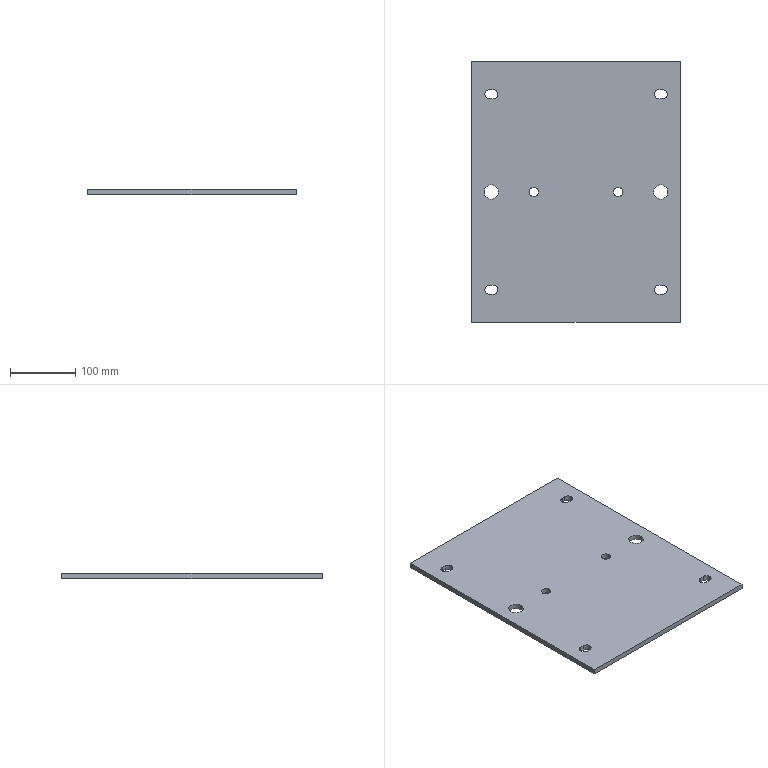Part | 1 solid | 34 faces | box 320 x 400 x 8 mm | volume 1007841 mm3 | cylinder 20 | plane 14 | commonest cylinder face diameters 14 x16 22 x4
STEP:
#1=CARTESIAN_POINT('',(140.,150.,-8.));
#2=VERTEX_POINT('',#1);
#3=CARTESIAN_POINT('',(133.,157.,-8.));
#4=VERTEX_POINT('',#3);
#5=CARTESIAN_POINT('',(133.,150.,-8.));
#6=DIRECTION('',(0.,0.,1.));
#7=DIRECTION('',(1.,0.,0.));
#8=AXIS2_PLACEMENT_3D('',#5,#6,#7);
#9=CIRCLE('',#8,7.);
#10=EDGE_CURVE('',#2,#4,#9,.T.);
#11=ORIENTED_EDGE('',*,*,#10,.F.);
#12=CARTESIAN_POINT('',(140.,150.,0.));
#13=VERTEX_POINT('',#12);
#14=CARTESIAN_POINT('',(140.,150.,-10.));
#15=DIRECTION('',(0.,0.,1.));
#16=VECTOR('',#15,1000.);
#17=LINE('',#14,#16);
#18=EDGE_CURVE('',#2,#13,#17,.T.);
#19=ORIENTED_EDGE('',*,*,#18,.T.);
#20=CARTESIAN_POINT('',(133.,157.,0.));
#21=VERTEX_POINT('',#20);
#22=CARTESIAN_POINT('',(133.,150.,0.));
#23=DIRECTION('',(0.,0.,1.));
#24=DIRECTION('',(-1.,0.,0.));
#25=AXIS2_PLACEMENT_3D('',#22,#23,#24);
#26=CIRCLE('',#25,7.);
#27=EDGE_CURVE('',#13,#21,#26,.T.);
#28=ORIENTED_EDGE('',*,*,#27,.T.);
#29=CARTESIAN_POINT('',(133.,157.,-10.));
#30=DIRECTION('',(0.,0.,1.));
#31=VECTOR('',#30,1000.);
#32=LINE('',#29,#31);
#33=EDGE_CURVE('',#4,#21,#32,.T.);
#34=ORIENTED_EDGE('',*,*,#33,.F.);
#35=EDGE_LOOP('',(#11,#19,#28,#34));
#36=FACE_OUTER_BOUND('',#35,.T.);
#37=CARTESIAN_POINT('',(133.,150.,-10.));
#38=DIRECTION('',(0.,0.,1.));
#39=DIRECTION('',(1.,0.,0.));
#40=AXIS2_PLACEMENT_3D('',#37,#38,#39);
#41=CYLINDRICAL_SURFACE('',#40,7.);
#42=ADVANCED_FACE('',(#36),#41,.F.);
#43=CARTESIAN_POINT('',(119.,0.,-8.));
#44=VERTEX_POINT('',#43);
#45=CARTESIAN_POINT('',(141.,0.,-8.));
#46=VERTEX_POINT('',#45);
#47=CARTESIAN_POINT('',(130.,0.,-8.));
#48=DIRECTION('',(0.,0.,1.));
#49=DIRECTION('',(1.,0.,0.));
#50=AXIS2_PLACEMENT_3D('',#47,#48,#49);
#51=CIRCLE('',#50,11.);
#52=EDGE_CURVE('',#44,#46,#51,.T.);
#53=ORIENTED_EDGE('',*,*,#52,.F.);
#54=CARTESIAN_POINT('',(119.,0.,0.));
#55=VERTEX_POINT('',#54);
#56=CARTESIAN_POINT('',(119.,0.,-10.));
#57=DIRECTION('',(0.,0.,1.));
#58=VECTOR('',#57,1000.);
#59=LINE('',#56,#58);
#60=EDGE_CURVE('',#44,#55,#59,.T.);
#61=ORIENTED_EDGE('',*,*,#60,.T.);
#62=CARTESIAN_POINT('',(141.,0.,0.));
#63=VERTEX_POINT('',#62);
#64=CARTESIAN_POINT('',(130.,0.,0.));
#65=DIRECTION('',(0.,0.,1.));
#66=DIRECTION('',(-1.,0.,0.));
#67=AXIS2_PLACEMENT_3D('',#64,#65,#66);
#68=CIRCLE('',#67,11.);
#69=EDGE_CURVE('',#55,#63,#68,.T.);
#70=ORIENTED_EDGE('',*,*,#69,.T.);
#71=CARTESIAN_POINT('',(141.,0.,-10.));
#72=DIRECTION('',(0.,0.,1.));
#73=VECTOR('',#72,1000.);
#74=LINE('',#71,#73);
#75=EDGE_CURVE('',#46,#63,#74,.T.);
#76=ORIENTED_EDGE('',*,*,#75,.F.);
#77=EDGE_LOOP('',(#53,#61,#70,#76));
#78=FACE_OUTER_BOUND('',#77,.T.);
#79=CARTESIAN_POINT('',(130.,0.,-10.));
#80=DIRECTION('',(0.,0.,1.));
#81=DIRECTION('',(1.,0.,0.));
#82=AXIS2_PLACEMENT_3D('',#79,#80,#81);
#83=CYLINDRICAL_SURFACE('',#82,11.);
#84=ADVANCED_FACE('',(#78),#83,.F.);
#85=CARTESIAN_POINT('',(140.,-150.,-8.));
#86=VERTEX_POINT('',#85);
#87=CARTESIAN_POINT('',(133.,-143.,-8.));
#88=VERTEX_POINT('',#87);
#89=CARTESIAN_POINT('',(133.,-150.,-8.));
#90=DIRECTION('',(0.,0.,1.));
#91=DIRECTION('',(1.,0.,0.));
#92=AXIS2_PLACEMENT_3D('',#89,#90,#91);
#93=CIRCLE('',#92,7.);
#94=EDGE_CURVE('',#86,#88,#93,.T.);
#95=ORIENTED_EDGE('',*,*,#94,.F.);
#96=CARTESIAN_POINT('',(140.,-150.,0.));
#97=VERTEX_POINT('',#96);
#98=CARTESIAN_POINT('',(140.,-150.,-10.));
#99=DIRECTION('',(0.,0.,1.));
#100=VECTOR('',#99,1000.);
#101=LINE('',#98,#100);
#102=EDGE_CURVE('',#86,#97,#101,.T.);
#103=ORIENTED_EDGE('',*,*,#102,.T.);
#104=CARTESIAN_POINT('',(133.,-143.,0.));
#105=VERTEX_POINT('',#104);
#106=CARTESIAN_POINT('',(133.,-150.,0.));
#107=DIRECTION('',(0.,0.,1.));
#108=DIRECTION('',(1.,0.,0.));
#109=AXIS2_PLACEMENT_3D('',#106,#107,#108);
#110=CIRCLE('',#109,7.);
#111=EDGE_CURVE('',#97,#105,#110,.T.);
#112=ORIENTED_EDGE('',*,*,#111,.T.);
#113=CARTESIAN_POINT('',(133.,-143.,-10.));
#114=DIRECTION('',(0.,0.,1.));
#115=VECTOR('',#114,1000.);
#116=LINE('',#113,#115);
#117=EDGE_CURVE('',#88,#105,#116,.T.);
#118=ORIENTED_EDGE('',*,*,#117,.F.);
#119=EDGE_LOOP('',(#95,#103,#112,#118));
#120=FACE_OUTER_BOUND('',#119,.T.);
#121=CARTESIAN_POINT('',(133.,-150.,-10.));
#122=DIRECTION('',(0.,0.,1.));
#123=DIRECTION('',(1.,0.,0.));
#124=AXIS2_PLACEMENT_3D('',#121,#122,#123);
#125=CYLINDRICAL_SURFACE('',#124,7.);
#126=ADVANCED_FACE('',(#120),#125,.F.);
#127=CARTESIAN_POINT('',(-141.,0.,-8.));
#128=VERTEX_POINT('',#127);
#129=CARTESIAN_POINT('',(-119.,0.,-8.));
#130=VERTEX_POINT('',#129);
#131=CARTESIAN_POINT('',(-130.,0.,-8.));
#132=DIRECTION('',(0.,0.,1.));
#133=DIRECTION('',(1.,0.,0.));
#134=AXIS2_PLACEMENT_3D('',#131,#132,#133);
#135=CIRCLE('',#134,11.);
#136=EDGE_CURVE('',#128,#130,#135,.T.);
#137=ORIENTED_EDGE('',*,*,#136,.F.);
#138=CARTESIAN_POINT('',(-141.,0.,0.));
#139=VERTEX_POINT('',#138);
#140=CARTESIAN_POINT('',(-141.,0.,-10.));
#141=DIRECTION('',(0.,0.,1.));
#142=VECTOR('',#141,1000.);
#143=LINE('',#140,#142);
#144=EDGE_CURVE('',#128,#139,#143,.T.);
#145=ORIENTED_EDGE('',*,*,#144,.T.);
#146=CARTESIAN_POINT('',(-119.,0.,0.));
#147=VERTEX_POINT('',#146);
#148=CARTESIAN_POINT('',(-130.,0.,0.));
#149=DIRECTION('',(0.,0.,1.));
#150=DIRECTION('',(1.,0.,0.));
#151=AXIS2_PLACEMENT_3D('',#148,#149,#150);
#152=CIRCLE('',#151,11.);
#153=EDGE_CURVE('',#139,#147,#152,.T.);
#154=ORIENTED_EDGE('',*,*,#153,.T.);
#155=CARTESIAN_POINT('',(-119.,0.,-10.));
#156=DIRECTION('',(0.,0.,1.));
#157=VECTOR('',#156,1000.);
#158=LINE('',#155,#157);
#159=EDGE_CURVE('',#130,#147,#158,.T.);
#160=ORIENTED_EDGE('',*,*,#159,.F.);
#161=EDGE_LOOP('',(#137,#145,#154,#160));
#162=FACE_OUTER_BOUND('',#161,.T.);
#163=CARTESIAN_POINT('',(-130.,0.,-10.));
#164=DIRECTION('',(0.,0.,1.));
#165=DIRECTION('',(1.,0.,0.));
#166=AXIS2_PLACEMENT_3D('',#163,#164,#165);
#167=CYLINDRICAL_SURFACE('',#166,11.);
#168=ADVANCED_FACE('',(#162),#167,.F.);
#169=CARTESIAN_POINT('',(-120.,150.,-8.));
#170=VERTEX_POINT('',#169);
#171=CARTESIAN_POINT('',(-127.,157.,-8.));
#172=VERTEX_POINT('',#171);
#173=CARTESIAN_POINT('',(-127.,150.,-8.));
#174=DIRECTION('',(0.,0.,1.));
#175=DIRECTION('',(1.,0.,0.));
#176=AXIS2_PLACEMENT_3D('',#173,#174,#175);
#177=CIRCLE('',#176,7.);
#178=EDGE_CURVE('',#170,#172,#177,.T.);
#179=ORIENTED_EDGE('',*,*,#178,.F.);
#180=CARTESIAN_POINT('',(-120.,150.,0.));
#181=VERTEX_POINT('',#180);
#182=CARTESIAN_POINT('',(-120.,150.,-10.));
#183=DIRECTION('',(0.,0.,1.));
#184=VECTOR('',#183,1000.);
#185=LINE('',#182,#184);
#186=EDGE_CURVE('',#170,#181,#185,.T.);
#187=ORIENTED_EDGE('',*,*,#186,.T.);
#188=CARTESIAN_POINT('',(-127.,157.,0.));
#189=VERTEX_POINT('',#188);
#190=CARTESIAN_POINT('',(-127.,150.,0.));
#191=DIRECTION('',(0.,0.,1.));
#192=DIRECTION('',(1.,0.,0.));
#193=AXIS2_PLACEMENT_3D('',#190,#191,#192);
#194=CIRCLE('',#193,7.);
#195=EDGE_CURVE('',#181,#189,#194,.T.);
#196=ORIENTED_EDGE('',*,*,#195,.T.);
#197=CARTESIAN_POINT('',(-127.,157.,-10.));
#198=DIRECTION('',(0.,0.,1.));
#199=VECTOR('',#198,1000.);
#200=LINE('',#197,#199);
#201=EDGE_CURVE('',#172,#189,#200,.T.);
#202=ORIENTED_EDGE('',*,*,#201,.F.);
#203=EDGE_LOOP('',(#179,#187,#196,#202));
#204=FACE_OUTER_BOUND('',#203,.T.);
#205=CARTESIAN_POINT('',(-127.,150.,-10.));
#206=DIRECTION('',(0.,0.,1.));
#207=DIRECTION('',(1.,0.,0.));
#208=AXIS2_PLACEMENT_3D('',#205,#206,#207);
#209=CYLINDRICAL_SURFACE('',#208,7.);
#210=ADVANCED_FACE('',(#204),#209,.F.);
#211=CARTESIAN_POINT('',(-120.,-150.,-8.));
#212=VERTEX_POINT('',#211);
#213=CARTESIAN_POINT('',(-127.,-143.,-8.));
#214=VERTEX_POINT('',#213);
#215=CARTESIAN_POINT('',(-127.,-150.,-8.));
#216=DIRECTION('',(0.,0.,1.));
#217=DIRECTION('',(1.,0.,0.));
#218=AXIS2_PLACEMENT_3D('',#215,#216,#217);
#219=CIRCLE('',#218,7.);
#220=EDGE_CURVE('',#212,#214,#219,.T.);
#221=ORIENTED_EDGE('',*,*,#220,.F.);
#222=CARTESIAN_POINT('',(-120.,-150.,0.));
#223=VERTEX_POINT('',#222);
#224=CARTESIAN_POINT('',(-120.,-150.,-10.));
#225=DIRECTION('',(0.,0.,1.));
#226=VECTOR('',#225,1000.);
#227=LINE('',#224,#226);
#228=EDGE_CURVE('',#212,#223,#227,.T.);
#229=ORIENTED_EDGE('',*,*,#228,.T.);
#230=CARTESIAN_POINT('',(-127.,-143.,0.));
#231=VERTEX_POINT('',#230);
#232=CARTESIAN_POINT('',(-127.,-150.,0.));
#233=DIRECTION('',(0.,0.,1.));
#234=DIRECTION('',(-1.,0.,0.));
#235=AXIS2_PLACEMENT_3D('',#232,#233,#234);
#236=CIRCLE('',#235,7.);
#237=EDGE_CURVE('',#223,#231,#236,.T.);
#238=ORIENTED_EDGE('',*,*,#237,.T.);
#239=CARTESIAN_POINT('',(-127.,-143.,-10.));
#240=DIRECTION('',(0.,0.,1.));
#241=VECTOR('',#240,1000.);
#242=LINE('',#239,#241);
#243=EDGE_CURVE('',#214,#231,#242,.T.);
#244=ORIENTED_EDGE('',*,*,#243,.F.);
#245=EDGE_LOOP('',(#221,#229,#238,#244));
#246=FACE_OUTER_BOUND('',#245,.T.);
#247=CARTESIAN_POINT('',(-127.,-150.,-10.));
#248=DIRECTION('',(0.,0.,1.));
#249=DIRECTION('',(1.,0.,0.));
#250=AXIS2_PLACEMENT_3D('',#247,#248,#249);
#251=CYLINDRICAL_SURFACE('',#250,7.);
#252=ADVANCED_FACE('',(#246),#251,.F.);
#253=CARTESIAN_POINT('',(58.,0.,-8.));
#254=VERTEX_POINT('',#253);
#255=CARTESIAN_POINT('',(72.,0.,-8.));
#256=VERTEX_POINT('',#255);
#257=CARTESIAN_POINT('',(65.,0.,-8.));
#258=DIRECTION('',(0.,0.,1.));
#259=DIRECTION('',(1.,0.,0.));
#260=AXIS2_PLACEMENT_3D('',#257,#258,#259);
#261=CIRCLE('',#260,7.);
#262=EDGE_CURVE('',#254,#256,#261,.T.);
#263=ORIENTED_EDGE('',*,*,#262,.F.);
#264=CARTESIAN_POINT('',(58.,0.,0.));
#265=VERTEX_POINT('',#264);
#266=CARTESIAN_POINT('',(58.,0.,-10.));
#267=DIRECTION('',(0.,0.,1.));
#268=VECTOR('',#267,1000.);
#269=LINE('',#266,#268);
#270=EDGE_CURVE('',#254,#265,#269,.T.);
#271=ORIENTED_EDGE('',*,*,#270,.T.);
#272=CARTESIAN_POINT('',(72.,0.,0.));
#273=VERTEX_POINT('',#272);
#274=CARTESIAN_POINT('',(65.,0.,0.));
#275=DIRECTION('',(0.,0.,1.));
#276=DIRECTION('',(-1.,0.,0.));
#277=AXIS2_PLACEMENT_3D('',#274,#275,#276);
#278=CIRCLE('',#277,7.);
#279=EDGE_CURVE('',#265,#273,#278,.T.);
#280=ORIENTED_EDGE('',*,*,#279,.T.);
#281=CARTESIAN_POINT('',(72.,0.,-10.));
#282=DIRECTION('',(0.,0.,1.));
#283=VECTOR('',#282,1000.);
#284=LINE('',#281,#283);
#285=EDGE_CURVE('',#256,#273,#284,.T.);
#286=ORIENTED_EDGE('',*,*,#285,.F.);
#287=EDGE_LOOP('',(#263,#271,#280,#286));
#288=FACE_OUTER_BOUND('',#287,.T.);
#289=CARTESIAN_POINT('',(65.,0.,-10.));
#290=DIRECTION('',(0.,0.,1.));
#291=DIRECTION('',(1.,0.,0.));
#292=AXIS2_PLACEMENT_3D('',#289,#290,#291);
#293=CYLINDRICAL_SURFACE('',#292,7.);
#294=ADVANCED_FACE('',(#288),#293,.F.);
#295=CARTESIAN_POINT('',(-72.,0.,-8.));
#296=VERTEX_POINT('',#295);
#297=CARTESIAN_POINT('',(-58.,0.,-8.));
#298=VERTEX_POINT('',#297);
#299=CARTESIAN_POINT('',(-65.,0.,-8.));
#300=DIRECTION('',(0.,0.,1.));
#301=DIRECTION('',(1.,0.,0.));
#302=AXIS2_PLACEMENT_3D('',#299,#300,#301);
#303=CIRCLE('',#302,7.);
#304=EDGE_CURVE('',#296,#298,#303,.T.);
#305=ORIENTED_EDGE('',*,*,#304,.F.);
#306=CARTESIAN_POINT('',(-72.,0.,0.));
#307=VERTEX_POINT('',#306);
#308=CARTESIAN_POINT('',(-72.,0.,-10.));
#309=DIRECTION('',(0.,0.,1.));
#310=VECTOR('',#309,1000.);
#311=LINE('',#308,#310);
#312=EDGE_CURVE('',#296,#307,#311,.T.);
#313=ORIENTED_EDGE('',*,*,#312,.T.);
#314=CARTESIAN_POINT('',(-58.,0.,0.));
#315=VERTEX_POINT('',#314);
#316=CARTESIAN_POINT('',(-65.,0.,0.));
#317=DIRECTION('',(0.,0.,1.));
#318=DIRECTION('',(1.,0.,0.));
#319=AXIS2_PLACEMENT_3D('',#316,#317,#318);
#320=CIRCLE('',#319,7.);
#321=EDGE_CURVE('',#307,#315,#320,.T.);
#322=ORIENTED_EDGE('',*,*,#321,.T.);
#323=CARTESIAN_POINT('',(-58.,0.,-10.));
#324=DIRECTION('',(0.,0.,1.));
#325=VECTOR('',#324,1000.);
#326=LINE('',#323,#325);
#327=EDGE_CURVE('',#298,#315,#326,.T.);
#328=ORIENTED_EDGE('',*,*,#327,.F.);
#329=EDGE_LOOP('',(#305,#313,#322,#328));
#330=FACE_OUTER_BOUND('',#329,.T.);
#331=CARTESIAN_POINT('',(-65.,0.,-10.));
#332=DIRECTION('',(0.,0.,1.));
#333=DIRECTION('',(1.,0.,0.));
#334=AXIS2_PLACEMENT_3D('',#331,#332,#333);
#335=CYLINDRICAL_SURFACE('',#334,7.);
#336=ADVANCED_FACE('',(#330),#335,.F.);
#337=CARTESIAN_POINT('',(160.,-200.,0.));
#338=VERTEX_POINT('',#337);
#339=CARTESIAN_POINT('',(160.,200.,0.));
#340=VERTEX_POINT('',#339);
#341=CARTESIAN_POINT('',(160.,200.,0.));
#342=DIRECTION('',(0.,1.,0.));
#343=VECTOR('',#342,1000.);
#344=LINE('',#341,#343);
#345=EDGE_CURVE('',#338,#340,#344,.T.);
#346=ORIENTED_EDGE('',*,*,#345,.F.);
#347=CARTESIAN_POINT('',(160.,-200.,-8.));
#348=VERTEX_POINT('',#347);
#349=CARTESIAN_POINT('',(160.,-200.,-8.));
#350=DIRECTION('',(0.,0.,1.));
#351=VECTOR('',#350,1000.);
#352=LINE('',#349,#351);
#353=EDGE_CURVE('',#348,#338,#352,.T.);
#354=ORIENTED_EDGE('',*,*,#353,.F.);
#355=CARTESIAN_POINT('',(160.,200.,-8.));
#356=VERTEX_POINT('',#355);
#357=CARTESIAN_POINT('',(160.,200.,-8.));
#358=DIRECTION('',(0.,1.,0.));
#359=VECTOR('',#358,1000.);
#360=LINE('',#357,#359);
#361=EDGE_CURVE('',#348,#356,#360,.T.);
#362=ORIENTED_EDGE('',*,*,#361,.T.);
#363=CARTESIAN_POINT('',(160.,200.,-8.));
#364=DIRECTION('',(0.,0.,1.));
#365=VECTOR('',#364,1000.);
#366=LINE('',#363,#365);
#367=EDGE_CURVE('',#356,#340,#366,.T.);
#368=ORIENTED_EDGE('',*,*,#367,.T.);
#369=EDGE_LOOP('',(#346,#354,#362,#368));
#370=FACE_OUTER_BOUND('',#369,.T.);
#371=CARTESIAN_POINT('',(160.,200.,-8.));
#372=DIRECTION('',(1.,0.,0.));
#373=DIRECTION('',(0.,1.,0.));
#374=AXIS2_PLACEMENT_3D('',#371,#372,#373);
#375=PLANE('',#374);
#376=ADVANCED_FACE('',(#370),#375,.T.);
#377=CARTESIAN_POINT('',(-160.,-200.,0.));
#378=VERTEX_POINT('',#377);
#379=CARTESIAN_POINT('',(-160.,-200.,0.));
#380=DIRECTION('',(1.,0.,0.));
#381=VECTOR('',#380,1000.);
#382=LINE('',#379,#381);
#383=EDGE_CURVE('',#378,#338,#382,.T.);
#384=ORIENTED_EDGE('',*,*,#383,.F.);
#385=CARTESIAN_POINT('',(-160.,-200.,-8.));
#386=VERTEX_POINT('',#385);
#387=CARTESIAN_POINT('',(-160.,-200.,-8.));
#388=DIRECTION('',(0.,0.,1.));
#389=VECTOR('',#388,1000.);
#390=LINE('',#387,#389);
#391=EDGE_CURVE('',#386,#378,#390,.T.);
#392=ORIENTED_EDGE('',*,*,#391,.F.);
#393=CARTESIAN_POINT('',(-160.,-200.,-8.));
#394=DIRECTION('',(1.,0.,0.));
#395=VECTOR('',#394,1000.);
#396=LINE('',#393,#395);
#397=EDGE_CURVE('',#386,#348,#396,.T.);
#398=ORIENTED_EDGE('',*,*,#397,.T.);
#399=ORIENTED_EDGE('',*,*,#353,.T.);
#400=EDGE_LOOP('',(#384,#392,#398,#399));
#401=FACE_OUTER_BOUND('',#400,.T.);
#402=CARTESIAN_POINT('',(-160.,-200.,-8.));
#403=DIRECTION('',(0.,-1.,0.));
#404=DIRECTION('',(0.,0.,-1.));
#405=AXIS2_PLACEMENT_3D('',#402,#403,#404);
#406=PLANE('',#405);
#407=ADVANCED_FACE('',(#401),#406,.T.);
#408=CARTESIAN_POINT('',(-160.,200.,0.));
#409=VERTEX_POINT('',#408);
#410=CARTESIAN_POINT('',(-160.,200.,0.));
#411=DIRECTION('',(0.,-1.,0.));
#412=VECTOR('',#411,1000.);
#413=LINE('',#410,#412);
#414=EDGE_CURVE('',#409,#378,#413,.T.);
#415=ORIENTED_EDGE('',*,*,#414,.F.);
#416=CARTESIAN_POINT('',(-160.,200.,-8.));
#417=VERTEX_POINT('',#416);
#418=CARTESIAN_POINT('',(-160.,200.,-8.));
#419=DIRECTION('',(0.,0.,1.));
#420=VECTOR('',#419,1000.);
#421=LINE('',#418,#420);
#422=EDGE_CURVE('',#417,#409,#421,.T.);
#423=ORIENTED_EDGE('',*,*,#422,.F.);
#424=CARTESIAN_POINT('',(-160.,200.,-8.));
#425=DIRECTION('',(0.,-1.,0.));
#426=VECTOR('',#425,1000.);
#427=LINE('',#424,#426);
#428=EDGE_CURVE('',#417,#386,#427,.T.);
#429=ORIENTED_EDGE('',*,*,#428,.T.);
#430=ORIENTED_EDGE('',*,*,#391,.T.);
#431=EDGE_LOOP('',(#415,#423,#429,#430));
#432=FACE_OUTER_BOUND('',#431,.T.);
#433=CARTESIAN_POINT('',(-160.,200.,-8.));
#434=DIRECTION('',(-1.,0.,0.));
#435=DIRECTION('',(0.,-1.,0.));
#436=AXIS2_PLACEMENT_3D('',#433,#434,#435);
#437=PLANE('',#436);
#438=ADVANCED_FACE('',(#432),#437,.T.);
#439=CARTESIAN_POINT('',(-160.,200.,0.));
#440=DIRECTION('',(-1.,0.,0.));
#441=VECTOR('',#440,1000.);
#442=LINE('',#439,#441);
#443=EDGE_CURVE('',#340,#409,#442,.T.);
#444=ORIENTED_EDGE('',*,*,#443,.F.);
#445=ORIENTED_EDGE('',*,*,#367,.F.);
#446=CARTESIAN_POINT('',(-160.,200.,-8.));
#447=DIRECTION('',(-1.,0.,0.));
#448=VECTOR('',#447,1000.);
#449=LINE('',#446,#448);
#450=EDGE_CURVE('',#356,#417,#449,.T.);
#451=ORIENTED_EDGE('',*,*,#450,.T.);
#452=ORIENTED_EDGE('',*,*,#422,.T.);
#453=EDGE_LOOP('',(#444,#445,#451,#452));
#454=FACE_OUTER_BOUND('',#453,.T.);
#455=CARTESIAN_POINT('',(-160.,200.,-8.));
#456=DIRECTION('',(0.,1.,0.));
#457=DIRECTION('',(0.,0.,1.));
#458=AXIS2_PLACEMENT_3D('',#455,#456,#457);
#459=PLANE('',#458);
#460=ADVANCED_FACE('',(#454),#459,.T.);
#461=CARTESIAN_POINT('',(127.,143.,-8.));
#462=VERTEX_POINT('',#461);
#463=CARTESIAN_POINT('',(133.,143.,-8.));
#464=VERTEX_POINT('',#463);
#465=CARTESIAN_POINT('',(0.,143.,-8.));
#466=DIRECTION('',(1.,0.,0.));
#467=VECTOR('',#466,1000.);
#468=LINE('',#465,#467);
#469=EDGE_CURVE('',#462,#464,#468,.T.);
#470=ORIENTED_EDGE('',*,*,#469,.T.);
#471=CARTESIAN_POINT('',(133.,150.,-8.));
#472=DIRECTION('',(0.,0.,1.));
#473=DIRECTION('',(1.,0.,0.));
#474=AXIS2_PLACEMENT_3D('',#471,#472,#473);
#475=CIRCLE('',#474,7.);
#476=EDGE_CURVE('',#464,#2,#475,.T.);
#477=ORIENTED_EDGE('',*,*,#476,.T.);
#478=ORIENTED_EDGE('',*,*,#10,.T.);
#479=CARTESIAN_POINT('',(127.,157.,-8.));
#480=VERTEX_POINT('',#479);
#481=CARTESIAN_POINT('',(0.,157.,-8.));
#482=DIRECTION('',(-1.,0.,0.));
#483=VECTOR('',#482,1000.);
#484=LINE('',#481,#483);
#485=EDGE_CURVE('',#4,#480,#484,.T.);
#486=ORIENTED_EDGE('',*,*,#485,.T.);
#487=CARTESIAN_POINT('',(127.,150.,-8.));
#488=DIRECTION('',(0.,0.,1.));
#489=DIRECTION('',(1.,0.,0.));
#490=AXIS2_PLACEMENT_3D('',#487,#488,#489);
#491=CIRCLE('',#490,7.);
#492=EDGE_CURVE('',#480,#462,#491,.T.);
#493=ORIENTED_EDGE('',*,*,#492,.T.);
#494=EDGE_LOOP('',(#470,#477,#478,#486,#493));
#495=FACE_BOUND('',#494,.T.);
#496=CARTESIAN_POINT('',(130.,0.,-8.));
#497=DIRECTION('',(0.,0.,1.));
#498=DIRECTION('',(1.,0.,0.));
#499=AXIS2_PLACEMENT_3D('',#496,#497,#498);
#500=CIRCLE('',#499,11.);
#501=EDGE_CURVE('',#46,#44,#500,.T.);
#502=ORIENTED_EDGE('',*,*,#501,.T.);
#503=ORIENTED_EDGE('',*,*,#52,.T.);
#504=EDGE_LOOP('',(#502,#503));
#505=FACE_BOUND('',#504,.T.);
#506=CARTESIAN_POINT('',(127.,-157.,-8.));
#507=VERTEX_POINT('',#506);
#508=CARTESIAN_POINT('',(133.,-157.,-8.));
#509=VERTEX_POINT('',#508);
#510=CARTESIAN_POINT('',(0.,-157.,-8.));
#511=DIRECTION('',(1.,0.,0.));
#512=VECTOR('',#511,1000.);
#513=LINE('',#510,#512);
#514=EDGE_CURVE('',#507,#509,#513,.T.);
#515=ORIENTED_EDGE('',*,*,#514,.T.);
#516=CARTESIAN_POINT('',(133.,-150.,-8.));
#517=DIRECTION('',(0.,0.,1.));
#518=DIRECTION('',(1.,0.,0.));
#519=AXIS2_PLACEMENT_3D('',#516,#517,#518);
#520=CIRCLE('',#519,7.);
#521=EDGE_CURVE('',#509,#86,#520,.T.);
#522=ORIENTED_EDGE('',*,*,#521,.T.);
#523=ORIENTED_EDGE('',*,*,#94,.T.);
#524=CARTESIAN_POINT('',(127.,-143.,-8.));
#525=VERTEX_POINT('',#524);
#526=CARTESIAN_POINT('',(0.,-143.,-8.));
#527=DIRECTION('',(-1.,0.,0.));
#528=VECTOR('',#527,1000.);
#529=LINE('',#526,#528);
#530=EDGE_CURVE('',#88,#525,#529,.T.);
#531=ORIENTED_EDGE('',*,*,#530,.T.);
#532=CARTESIAN_POINT('',(127.,-150.,-8.));
#533=DIRECTION('',(0.,0.,1.));
#534=DIRECTION('',(1.,0.,0.));
#535=AXIS2_PLACEMENT_3D('',#532,#533,#534);
#536=CIRCLE('',#535,7.);
#537=EDGE_CURVE('',#525,#507,#536,.T.);
#538=ORIENTED_EDGE('',*,*,#537,.T.);
#539=EDGE_LOOP('',(#515,#522,#523,#531,#538));
#540=FACE_BOUND('',#539,.T.);
#541=CARTESIAN_POINT('',(-130.,0.,-8.));
#542=DIRECTION('',(0.,0.,1.));
#543=DIRECTION('',(1.,0.,0.));
#544=AXIS2_PLACEMENT_3D('',#541,#542,#543);
#545=CIRCLE('',#544,11.);
#546=EDGE_CURVE('',#130,#128,#545,.T.);
#547=ORIENTED_EDGE('',*,*,#546,.T.);
#548=ORIENTED_EDGE('',*,*,#136,.T.);
#549=EDGE_LOOP('',(#547,#548));
#550=FACE_BOUND('',#549,.T.);
#551=CARTESIAN_POINT('',(-133.,157.,-8.));
#552=VERTEX_POINT('',#551);
#553=CARTESIAN_POINT('',(0.,157.,-8.));
#554=DIRECTION('',(-1.,0.,0.));
#555=VECTOR('',#554,1000.);
#556=LINE('',#553,#555);
#557=EDGE_CURVE('',#172,#552,#556,.T.);
#558=ORIENTED_EDGE('',*,*,#557,.T.);
#559=CARTESIAN_POINT('',(-133.,143.,-8.));
#560=VERTEX_POINT('',#559);
#561=CARTESIAN_POINT('',(-133.,150.,-8.));
#562=DIRECTION('',(0.,0.,1.));
#563=DIRECTION('',(1.,0.,0.));
#564=AXIS2_PLACEMENT_3D('',#561,#562,#563);
#565=CIRCLE('',#564,7.);
#566=EDGE_CURVE('',#552,#560,#565,.T.);
#567=ORIENTED_EDGE('',*,*,#566,.T.);
#568=CARTESIAN_POINT('',(-127.,143.,-8.));
#569=VERTEX_POINT('',#568);
#570=CARTESIAN_POINT('',(0.,143.,-8.));
#571=DIRECTION('',(1.,0.,0.));
#572=VECTOR('',#571,1000.);
#573=LINE('',#570,#572);
#574=EDGE_CURVE('',#560,#569,#573,.T.);
#575=ORIENTED_EDGE('',*,*,#574,.T.);
#576=CARTESIAN_POINT('',(-127.,150.,-8.));
#577=DIRECTION('',(0.,0.,1.));
#578=DIRECTION('',(1.,0.,0.));
#579=AXIS2_PLACEMENT_3D('',#576,#577,#578);
#580=CIRCLE('',#579,7.);
#581=EDGE_CURVE('',#569,#170,#580,.T.);
#582=ORIENTED_EDGE('',*,*,#581,.T.);
#583=ORIENTED_EDGE('',*,*,#178,.T.);
#584=EDGE_LOOP('',(#558,#567,#575,#582,#583));
#585=FACE_BOUND('',#584,.T.);
#586=CARTESIAN_POINT('',(-133.,-143.,-8.));
#587=VERTEX_POINT('',#586);
#588=CARTESIAN_POINT('',(0.,-143.,-8.));
#589=DIRECTION('',(-1.,0.,0.));
#590=VECTOR('',#589,1000.);
#591=LINE('',#588,#590);
#592=EDGE_CURVE('',#214,#587,#591,.T.);
#593=ORIENTED_EDGE('',*,*,#592,.T.);
#594=CARTESIAN_POINT('',(-133.,-157.,-8.));
#595=VERTEX_POINT('',#594);
#596=CARTESIAN_POINT('',(-133.,-150.,-8.));
#597=DIRECTION('',(0.,0.,1.));
#598=DIRECTION('',(1.,0.,0.));
#599=AXIS2_PLACEMENT_3D('',#596,#597,#598);
#600=CIRCLE('',#599,7.);
#601=EDGE_CURVE('',#587,#595,#600,.T.);
#602=ORIENTED_EDGE('',*,*,#601,.T.);
#603=CARTESIAN_POINT('',(-127.,-157.,-8.));
#604=VERTEX_POINT('',#603);
#605=CARTESIAN_POINT('',(0.,-157.,-8.));
#606=DIRECTION('',(1.,0.,0.));
#607=VECTOR('',#606,1000.);
#608=LINE('',#605,#607);
#609=EDGE_CURVE('',#595,#604,#608,.T.);
#610=ORIENTED_EDGE('',*,*,#609,.T.);
#611=CARTESIAN_POINT('',(-127.,-150.,-8.));
#612=DIRECTION('',(0.,0.,1.));
#613=DIRECTION('',(1.,0.,0.));
#614=AXIS2_PLACEMENT_3D('',#611,#612,#613);
#615=CIRCLE('',#614,7.);
#616=EDGE_CURVE('',#604,#212,#615,.T.);
#617=ORIENTED_EDGE('',*,*,#616,.T.);
#618=ORIENTED_EDGE('',*,*,#220,.T.);
#619=EDGE_LOOP('',(#593,#602,#610,#617,#618));
#620=FACE_BOUND('',#619,.T.);
#621=CARTESIAN_POINT('',(65.,0.,-8.));
#622=DIRECTION('',(0.,0.,1.));
#623=DIRECTION('',(1.,0.,0.));
#624=AXIS2_PLACEMENT_3D('',#621,#622,#623);
#625=CIRCLE('',#624,7.);
#626=EDGE_CURVE('',#256,#254,#625,.T.);
#627=ORIENTED_EDGE('',*,*,#626,.T.);
#628=ORIENTED_EDGE('',*,*,#262,.T.);
#629=EDGE_LOOP('',(#627,#628));
#630=FACE_BOUND('',#629,.T.);
#631=CARTESIAN_POINT('',(-65.,0.,-8.));
#632=DIRECTION('',(0.,0.,1.));
#633=DIRECTION('',(1.,0.,0.));
#634=AXIS2_PLACEMENT_3D('',#631,#632,#633);
#635=CIRCLE('',#634,7.);
#636=EDGE_CURVE('',#298,#296,#635,.T.);
#637=ORIENTED_EDGE('',*,*,#636,.T.);
#638=ORIENTED_EDGE('',*,*,#304,.T.);
#639=EDGE_LOOP('',(#637,#638));
#640=FACE_BOUND('',#639,.T.);
#641=ORIENTED_EDGE('',*,*,#361,.F.);
#642=ORIENTED_EDGE('',*,*,#397,.F.);
#643=ORIENTED_EDGE('',*,*,#428,.F.);
#644=ORIENTED_EDGE('',*,*,#450,.F.);
#645=EDGE_LOOP('',(#641,#642,#643,#644));
#646=FACE_OUTER_BOUND('',#645,.T.);
#647=CARTESIAN_POINT('',(0.,0.,-8.));
#648=DIRECTION('',(0.,0.,1.));
#649=DIRECTION('',(1.,0.,0.));
#650=AXIS2_PLACEMENT_3D('',#647,#648,#649);
#651=PLANE('',#650);
#652=ADVANCED_FACE('',(#495,#505,#540,#550,#585,#620,#630,#640,#646),#651,.F.);
#653=CARTESIAN_POINT('',(133.,143.,0.));
#654=VERTEX_POINT('',#653);
#655=CARTESIAN_POINT('',(133.,150.,0.));
#656=DIRECTION('',(0.,0.,1.));
#657=DIRECTION('',(-1.,0.,0.));
#658=AXIS2_PLACEMENT_3D('',#655,#656,#657);
#659=CIRCLE('',#658,7.);
#660=EDGE_CURVE('',#654,#13,#659,.T.);
#661=ORIENTED_EDGE('',*,*,#660,.F.);
#662=CARTESIAN_POINT('',(127.,143.,0.));
#663=VERTEX_POINT('',#662);
#664=CARTESIAN_POINT('',(133.,143.,0.));
#665=DIRECTION('',(1.,0.,0.));
#666=VECTOR('',#665,1000.);
#667=LINE('',#664,#666);
#668=EDGE_CURVE('',#663,#654,#667,.T.);
#669=ORIENTED_EDGE('',*,*,#668,.F.);
#670=CARTESIAN_POINT('',(127.,157.,0.));
#671=VERTEX_POINT('',#670);
#672=CARTESIAN_POINT('',(127.,150.,0.));
#673=DIRECTION('',(0.,0.,1.));
#674=DIRECTION('',(-1.,0.,0.));
#675=AXIS2_PLACEMENT_3D('',#672,#673,#674);
#676=CIRCLE('',#675,7.);
#677=EDGE_CURVE('',#671,#663,#676,.T.);
#678=ORIENTED_EDGE('',*,*,#677,.F.);
#679=CARTESIAN_POINT('',(133.,157.,0.));
#680=DIRECTION('',(-1.,0.,0.));
#681=VECTOR('',#680,1000.);
#682=LINE('',#679,#681);
#683=EDGE_CURVE('',#21,#671,#682,.T.);
#684=ORIENTED_EDGE('',*,*,#683,.F.);
#685=ORIENTED_EDGE('',*,*,#27,.F.);
#686=EDGE_LOOP('',(#661,#669,#678,#684,#685));
#687=FACE_BOUND('',#686,.T.);
#688=CARTESIAN_POINT('',(130.,0.,0.));
#689=DIRECTION('',(0.,0.,1.));
#690=DIRECTION('',(-1.,0.,0.));
#691=AXIS2_PLACEMENT_3D('',#688,#689,#690);
#692=CIRCLE('',#691,11.);
#693=EDGE_CURVE('',#63,#55,#692,.T.);
#694=ORIENTED_EDGE('',*,*,#693,.F.);
#695=ORIENTED_EDGE('',*,*,#69,.F.);
#696=EDGE_LOOP('',(#694,#695));
#697=FACE_BOUND('',#696,.T.);
#698=CARTESIAN_POINT('',(133.,-157.,0.));
#699=VERTEX_POINT('',#698);
#700=CARTESIAN_POINT('',(133.,-150.,0.));
#701=DIRECTION('',(0.,0.,1.));
#702=DIRECTION('',(1.,0.,0.));
#703=AXIS2_PLACEMENT_3D('',#700,#701,#702);
#704=CIRCLE('',#703,7.);
#705=EDGE_CURVE('',#699,#97,#704,.T.);
#706=ORIENTED_EDGE('',*,*,#705,.F.);
#707=CARTESIAN_POINT('',(127.,-157.,0.));
#708=VERTEX_POINT('',#707);
#709=CARTESIAN_POINT('',(133.,-157.,0.));
#710=DIRECTION('',(1.,0.,0.));
#711=VECTOR('',#710,1000.);
#712=LINE('',#709,#711);
#713=EDGE_CURVE('',#708,#699,#712,.T.);
#714=ORIENTED_EDGE('',*,*,#713,.F.);
#715=CARTESIAN_POINT('',(127.,-143.,0.));
#716=VERTEX_POINT('',#715);
#717=CARTESIAN_POINT('',(127.,-150.,0.));
#718=DIRECTION('',(0.,0.,1.));
#719=DIRECTION('',(1.,0.,0.));
#720=AXIS2_PLACEMENT_3D('',#717,#718,#719);
#721=CIRCLE('',#720,7.);
#722=EDGE_CURVE('',#716,#708,#721,.T.);
#723=ORIENTED_EDGE('',*,*,#722,.F.);
#724=CARTESIAN_POINT('',(133.,-143.,0.));
#725=DIRECTION('',(-1.,0.,0.));
#726=VECTOR('',#725,1000.);
#727=LINE('',#724,#726);
#728=EDGE_CURVE('',#105,#716,#727,.T.);
#729=ORIENTED_EDGE('',*,*,#728,.F.);
#730=ORIENTED_EDGE('',*,*,#111,.F.);
#731=EDGE_LOOP('',(#706,#714,#723,#729,#730));
#732=FACE_BOUND('',#731,.T.);
#733=CARTESIAN_POINT('',(-130.,0.,0.));
#734=DIRECTION('',(0.,0.,1.));
#735=DIRECTION('',(1.,0.,0.));
#736=AXIS2_PLACEMENT_3D('',#733,#734,#735);
#737=CIRCLE('',#736,11.);
#738=EDGE_CURVE('',#147,#139,#737,.T.);
#739=ORIENTED_EDGE('',*,*,#738,.F.);
#740=ORIENTED_EDGE('',*,*,#153,.F.);
#741=EDGE_LOOP('',(#739,#740));
#742=FACE_BOUND('',#741,.T.);
#743=CARTESIAN_POINT('',(-133.,157.,0.));
#744=VERTEX_POINT('',#743);
#745=CARTESIAN_POINT('',(-133.,143.,0.));
#746=VERTEX_POINT('',#745);
#747=CARTESIAN_POINT('',(-133.,150.,0.));
#748=DIRECTION('',(0.,0.,1.));
#749=DIRECTION('',(1.,0.,0.));
#750=AXIS2_PLACEMENT_3D('',#747,#748,#749);
#751=CIRCLE('',#750,7.);
#752=EDGE_CURVE('',#744,#746,#751,.T.);
#753=ORIENTED_EDGE('',*,*,#752,.F.);
#754=CARTESIAN_POINT('',(-133.,157.,0.));
#755=DIRECTION('',(-1.,0.,0.));
#756=VECTOR('',#755,1000.);
#757=LINE('',#754,#756);
#758=EDGE_CURVE('',#189,#744,#757,.T.);
#759=ORIENTED_EDGE('',*,*,#758,.F.);
#760=ORIENTED_EDGE('',*,*,#195,.F.);
#761=CARTESIAN_POINT('',(-127.,143.,0.));
#762=VERTEX_POINT('',#761);
#763=CARTESIAN_POINT('',(-127.,150.,0.));
#764=DIRECTION('',(0.,0.,1.));
#765=DIRECTION('',(1.,0.,0.));
#766=AXIS2_PLACEMENT_3D('',#763,#764,#765);
#767=CIRCLE('',#766,7.);
#768=EDGE_CURVE('',#762,#181,#767,.T.);
#769=ORIENTED_EDGE('',*,*,#768,.F.);
#770=CARTESIAN_POINT('',(-133.,143.,0.));
#771=DIRECTION('',(1.,0.,0.));
#772=VECTOR('',#771,1000.);
#773=LINE('',#770,#772);
#774=EDGE_CURVE('',#746,#762,#773,.T.);
#775=ORIENTED_EDGE('',*,*,#774,.F.);
#776=EDGE_LOOP('',(#753,#759,#760,#769,#775));
#777=FACE_BOUND('',#776,.T.);
#778=CARTESIAN_POINT('',(-133.,-143.,0.));
#779=VERTEX_POINT('',#778);
#780=CARTESIAN_POINT('',(-133.,-157.,0.));
#781=VERTEX_POINT('',#780);
#782=CARTESIAN_POINT('',(-133.,-150.,0.));
#783=DIRECTION('',(0.,0.,1.));
#784=DIRECTION('',(-1.,0.,0.));
#785=AXIS2_PLACEMENT_3D('',#782,#783,#784);
#786=CIRCLE('',#785,7.);
#787=EDGE_CURVE('',#779,#781,#786,.T.);
#788=ORIENTED_EDGE('',*,*,#787,.F.);
#789=CARTESIAN_POINT('',(-133.,-143.,0.));
#790=DIRECTION('',(-1.,0.,0.));
#791=VECTOR('',#790,1000.);
#792=LINE('',#789,#791);
#793=EDGE_CURVE('',#231,#779,#792,.T.);
#794=ORIENTED_EDGE('',*,*,#793,.F.);
#795=ORIENTED_EDGE('',*,*,#237,.F.);
#796=CARTESIAN_POINT('',(-127.,-157.,0.));
#797=VERTEX_POINT('',#796);
#798=CARTESIAN_POINT('',(-127.,-150.,0.));
#799=DIRECTION('',(0.,0.,1.));
#800=DIRECTION('',(-1.,0.,0.));
#801=AXIS2_PLACEMENT_3D('',#798,#799,#800);
#802=CIRCLE('',#801,7.);
#803=EDGE_CURVE('',#797,#223,#802,.T.);
#804=ORIENTED_EDGE('',*,*,#803,.F.);
#805=CARTESIAN_POINT('',(-133.,-157.,0.));
#806=DIRECTION('',(1.,0.,0.));
#807=VECTOR('',#806,1000.);
#808=LINE('',#805,#807);
#809=EDGE_CURVE('',#781,#797,#808,.T.);
#810=ORIENTED_EDGE('',*,*,#809,.F.);
#811=EDGE_LOOP('',(#788,#794,#795,#804,#810));
#812=FACE_BOUND('',#811,.T.);
#813=CARTESIAN_POINT('',(65.,0.,0.));
#814=DIRECTION('',(0.,0.,1.));
#815=DIRECTION('',(-1.,0.,0.));
#816=AXIS2_PLACEMENT_3D('',#813,#814,#815);
#817=CIRCLE('',#816,7.);
#818=EDGE_CURVE('',#273,#265,#817,.T.);
#819=ORIENTED_EDGE('',*,*,#818,.F.);
#820=ORIENTED_EDGE('',*,*,#279,.F.);
#821=EDGE_LOOP('',(#819,#820));
#822=FACE_BOUND('',#821,.T.);
#823=CARTESIAN_POINT('',(-65.,0.,0.));
#824=DIRECTION('',(0.,0.,1.));
#825=DIRECTION('',(1.,0.,0.));
#826=AXIS2_PLACEMENT_3D('',#823,#824,#825);
#827=CIRCLE('',#826,7.);
#828=EDGE_CURVE('',#315,#307,#827,.T.);
#829=ORIENTED_EDGE('',*,*,#828,.F.);
#830=ORIENTED_EDGE('',*,*,#321,.F.);
#831=EDGE_LOOP('',(#829,#830));
#832=FACE_BOUND('',#831,.T.);
#833=ORIENTED_EDGE('',*,*,#345,.T.);
#834=ORIENTED_EDGE('',*,*,#443,.T.);
#835=ORIENTED_EDGE('',*,*,#414,.T.);
#836=ORIENTED_EDGE('',*,*,#383,.T.);
#837=EDGE_LOOP('',(#833,#834,#835,#836));
#838=FACE_OUTER_BOUND('',#837,.T.);
#839=CARTESIAN_POINT('',(0.,0.,0.));
#840=DIRECTION('',(0.,0.,1.));
#841=DIRECTION('',(1.,0.,0.));
#842=AXIS2_PLACEMENT_3D('',#839,#840,#841);
#843=PLANE('',#842);
#844=ADVANCED_FACE('',(#687,#697,#732,#742,#777,#812,#822,#832,#838),#843,.T.);
#845=ORIENTED_EDGE('',*,*,#312,.F.);
#846=ORIENTED_EDGE('',*,*,#636,.F.);
#847=ORIENTED_EDGE('',*,*,#327,.T.);
#848=ORIENTED_EDGE('',*,*,#828,.T.);
#849=EDGE_LOOP('',(#845,#846,#847,#848));
#850=FACE_OUTER_BOUND('',#849,.T.);
#851=CARTESIAN_POINT('',(-65.,0.,-10.));
#852=DIRECTION('',(0.,0.,1.));
#853=DIRECTION('',(1.,0.,0.));
#854=AXIS2_PLACEMENT_3D('',#851,#852,#853);
#855=CYLINDRICAL_SURFACE('',#854,7.);
#856=ADVANCED_FACE('',(#850),#855,.F.);
#857=ORIENTED_EDGE('',*,*,#270,.F.);
#858=ORIENTED_EDGE('',*,*,#626,.F.);
#859=ORIENTED_EDGE('',*,*,#285,.T.);
#860=ORIENTED_EDGE('',*,*,#818,.T.);
#861=EDGE_LOOP('',(#857,#858,#859,#860));
#862=FACE_OUTER_BOUND('',#861,.T.);
#863=CARTESIAN_POINT('',(65.,0.,-10.));
#864=DIRECTION('',(0.,0.,1.));
#865=DIRECTION('',(1.,0.,0.));
#866=AXIS2_PLACEMENT_3D('',#863,#864,#865);
#867=CYLINDRICAL_SURFACE('',#866,7.);
#868=ADVANCED_FACE('',(#862),#867,.F.);
#869=CARTESIAN_POINT('',(-133.,-143.,-10.));
#870=DIRECTION('',(0.,0.,1.));
#871=VECTOR('',#870,1000.);
#872=LINE('',#869,#871);
#873=EDGE_CURVE('',#587,#779,#872,.T.);
#874=ORIENTED_EDGE('',*,*,#873,.T.);
#875=ORIENTED_EDGE('',*,*,#787,.T.);
#876=CARTESIAN_POINT('',(-133.,-157.,-10.));
#877=DIRECTION('',(0.,0.,1.));
#878=VECTOR('',#877,1000.);
#879=LINE('',#876,#878);
#880=EDGE_CURVE('',#595,#781,#879,.T.);
#881=ORIENTED_EDGE('',*,*,#880,.F.);
#882=ORIENTED_EDGE('',*,*,#601,.F.);
#883=EDGE_LOOP('',(#874,#875,#881,#882));
#884=FACE_OUTER_BOUND('',#883,.T.);
#885=CARTESIAN_POINT('',(-133.,-150.,-10.));
#886=DIRECTION('',(0.,0.,1.));
#887=DIRECTION('',(1.,0.,0.));
#888=AXIS2_PLACEMENT_3D('',#885,#886,#887);
#889=CYLINDRICAL_SURFACE('',#888,7.);
#890=ADVANCED_FACE('',(#884),#889,.F.);
#891=ORIENTED_EDGE('',*,*,#243,.T.);
#892=ORIENTED_EDGE('',*,*,#793,.T.);
#893=ORIENTED_EDGE('',*,*,#873,.F.);
#894=ORIENTED_EDGE('',*,*,#592,.F.);
#895=EDGE_LOOP('',(#891,#892,#893,#894));
#896=FACE_OUTER_BOUND('',#895,.T.);
#897=CARTESIAN_POINT('',(-133.,-143.,-10.));
#898=DIRECTION('',(0.,1.,0.));
#899=DIRECTION('',(0.,0.,1.));
#900=AXIS2_PLACEMENT_3D('',#897,#898,#899);
#901=PLANE('',#900);
#902=ADVANCED_FACE('',(#896),#901,.F.);
#903=ORIENTED_EDGE('',*,*,#228,.F.);
#904=ORIENTED_EDGE('',*,*,#616,.F.);
#905=CARTESIAN_POINT('',(-127.,-157.,-10.));
#906=DIRECTION('',(0.,0.,1.));
#907=VECTOR('',#906,1000.);
#908=LINE('',#905,#907);
#909=EDGE_CURVE('',#604,#797,#908,.T.);
#910=ORIENTED_EDGE('',*,*,#909,.T.);
#911=ORIENTED_EDGE('',*,*,#803,.T.);
#912=EDGE_LOOP('',(#903,#904,#910,#911));
#913=FACE_OUTER_BOUND('',#912,.T.);
#914=CARTESIAN_POINT('',(-127.,-150.,-10.));
#915=DIRECTION('',(0.,0.,1.));
#916=DIRECTION('',(1.,0.,0.));
#917=AXIS2_PLACEMENT_3D('',#914,#915,#916);
#918=CYLINDRICAL_SURFACE('',#917,7.);
#919=ADVANCED_FACE('',(#913),#918,.F.);
#920=ORIENTED_EDGE('',*,*,#880,.T.);
#921=ORIENTED_EDGE('',*,*,#809,.T.);
#922=ORIENTED_EDGE('',*,*,#909,.F.);
#923=ORIENTED_EDGE('',*,*,#609,.F.);
#924=EDGE_LOOP('',(#920,#921,#922,#923));
#925=FACE_OUTER_BOUND('',#924,.T.);
#926=CARTESIAN_POINT('',(-133.,-157.,-10.));
#927=DIRECTION('',(0.,-1.,0.));
#928=DIRECTION('',(0.,0.,-1.));
#929=AXIS2_PLACEMENT_3D('',#926,#927,#928);
#930=PLANE('',#929);
#931=ADVANCED_FACE('',(#925),#930,.F.);
#932=CARTESIAN_POINT('',(-133.,157.,-10.));
#933=DIRECTION('',(0.,0.,1.));
#934=VECTOR('',#933,1000.);
#935=LINE('',#932,#934);
#936=EDGE_CURVE('',#552,#744,#935,.T.);
#937=ORIENTED_EDGE('',*,*,#936,.T.);
#938=ORIENTED_EDGE('',*,*,#752,.T.);
#939=CARTESIAN_POINT('',(-133.,143.,-10.));
#940=DIRECTION('',(0.,0.,1.));
#941=VECTOR('',#940,1000.);
#942=LINE('',#939,#941);
#943=EDGE_CURVE('',#560,#746,#942,.T.);
#944=ORIENTED_EDGE('',*,*,#943,.F.);
#945=ORIENTED_EDGE('',*,*,#566,.F.);
#946=EDGE_LOOP('',(#937,#938,#944,#945));
#947=FACE_OUTER_BOUND('',#946,.T.);
#948=CARTESIAN_POINT('',(-133.,150.,-10.));
#949=DIRECTION('',(0.,0.,1.));
#950=DIRECTION('',(1.,0.,0.));
#951=AXIS2_PLACEMENT_3D('',#948,#949,#950);
#952=CYLINDRICAL_SURFACE('',#951,7.);
#953=ADVANCED_FACE('',(#947),#952,.F.);
#954=ORIENTED_EDGE('',*,*,#201,.T.);
#955=ORIENTED_EDGE('',*,*,#758,.T.);
#956=ORIENTED_EDGE('',*,*,#936,.F.);
#957=ORIENTED_EDGE('',*,*,#557,.F.);
#958=EDGE_LOOP('',(#954,#955,#956,#957));
#959=FACE_OUTER_BOUND('',#958,.T.);
#960=CARTESIAN_POINT('',(-133.,157.,-10.));
#961=DIRECTION('',(0.,1.,0.));
#962=DIRECTION('',(0.,0.,1.));
#963=AXIS2_PLACEMENT_3D('',#960,#961,#962);
#964=PLANE('',#963);
#965=ADVANCED_FACE('',(#959),#964,.F.);
#966=ORIENTED_EDGE('',*,*,#186,.F.);
#967=ORIENTED_EDGE('',*,*,#581,.F.);
#968=CARTESIAN_POINT('',(-127.,143.,-10.));
#969=DIRECTION('',(0.,0.,1.));
#970=VECTOR('',#969,1000.);
#971=LINE('',#968,#970);
#972=EDGE_CURVE('',#569,#762,#971,.T.);
#973=ORIENTED_EDGE('',*,*,#972,.T.);
#974=ORIENTED_EDGE('',*,*,#768,.T.);
#975=EDGE_LOOP('',(#966,#967,#973,#974));
#976=FACE_OUTER_BOUND('',#975,.T.);
#977=CARTESIAN_POINT('',(-127.,150.,-10.));
#978=DIRECTION('',(0.,0.,1.));
#979=DIRECTION('',(1.,0.,0.));
#980=AXIS2_PLACEMENT_3D('',#977,#978,#979);
#981=CYLINDRICAL_SURFACE('',#980,7.);
#982=ADVANCED_FACE('',(#976),#981,.F.);
#983=ORIENTED_EDGE('',*,*,#943,.T.);
#984=ORIENTED_EDGE('',*,*,#774,.T.);
#985=ORIENTED_EDGE('',*,*,#972,.F.);
#986=ORIENTED_EDGE('',*,*,#574,.F.);
#987=EDGE_LOOP('',(#983,#984,#985,#986));
#988=FACE_OUTER_BOUND('',#987,.T.);
#989=CARTESIAN_POINT('',(-133.,143.,-10.));
#990=DIRECTION('',(0.,-1.,0.));
#991=DIRECTION('',(0.,0.,-1.));
#992=AXIS2_PLACEMENT_3D('',#989,#990,#991);
#993=PLANE('',#992);
#994=ADVANCED_FACE('',(#988),#993,.F.);
#995=ORIENTED_EDGE('',*,*,#144,.F.);
#996=ORIENTED_EDGE('',*,*,#546,.F.);
#997=ORIENTED_EDGE('',*,*,#159,.T.);
#998=ORIENTED_EDGE('',*,*,#738,.T.);
#999=EDGE_LOOP('',(#995,#996,#997,#998));
#1000=FACE_OUTER_BOUND('',#999,.T.);
#1001=CARTESIAN_POINT('',(-130.,0.,-10.));
#1002=DIRECTION('',(0.,0.,1.));
#1003=DIRECTION('',(1.,0.,0.));
#1004=AXIS2_PLACEMENT_3D('',#1001,#1002,#1003);
#1005=CYLINDRICAL_SURFACE('',#1004,11.);
#1006=ADVANCED_FACE('',(#1000),#1005,.F.);
#1007=ORIENTED_EDGE('',*,*,#102,.F.);
#1008=ORIENTED_EDGE('',*,*,#521,.F.);
#1009=CARTESIAN_POINT('',(133.,-157.,-10.));
#1010=DIRECTION('',(0.,0.,1.));
#1011=VECTOR('',#1010,1000.);
#1012=LINE('',#1009,#1011);
#1013=EDGE_CURVE('',#509,#699,#1012,.T.);
#1014=ORIENTED_EDGE('',*,*,#1013,.T.);
#1015=ORIENTED_EDGE('',*,*,#705,.T.);
#1016=EDGE_LOOP('',(#1007,#1008,#1014,#1015));
#1017=FACE_OUTER_BOUND('',#1016,.T.);
#1018=CARTESIAN_POINT('',(133.,-150.,-10.));
#1019=DIRECTION('',(0.,0.,1.));
#1020=DIRECTION('',(1.,0.,0.));
#1021=AXIS2_PLACEMENT_3D('',#1018,#1019,#1020);
#1022=CYLINDRICAL_SURFACE('',#1021,7.);
#1023=ADVANCED_FACE('',(#1017),#1022,.F.);
#1024=CARTESIAN_POINT('',(127.,-157.,-10.));
#1025=DIRECTION('',(0.,0.,1.));
#1026=VECTOR('',#1025,1000.);
#1027=LINE('',#1024,#1026);
#1028=EDGE_CURVE('',#507,#708,#1027,.T.);
#1029=ORIENTED_EDGE('',*,*,#1028,.T.);
#1030=ORIENTED_EDGE('',*,*,#713,.T.);
#1031=ORIENTED_EDGE('',*,*,#1013,.F.);
#1032=ORIENTED_EDGE('',*,*,#514,.F.);
#1033=EDGE_LOOP('',(#1029,#1030,#1031,#1032));
#1034=FACE_OUTER_BOUND('',#1033,.T.);
#1035=CARTESIAN_POINT('',(133.,-157.,-10.));
#1036=DIRECTION('',(0.,-1.,0.));
#1037=DIRECTION('',(0.,0.,-1.));
#1038=AXIS2_PLACEMENT_3D('',#1035,#1036,#1037);
#1039=PLANE('',#1038);
#1040=ADVANCED_FACE('',(#1034),#1039,.F.);
#1041=CARTESIAN_POINT('',(127.,-143.,-10.));
#1042=DIRECTION('',(0.,0.,1.));
#1043=VECTOR('',#1042,1000.);
#1044=LINE('',#1041,#1043);
#1045=EDGE_CURVE('',#525,#716,#1044,.T.);
#1046=ORIENTED_EDGE('',*,*,#1045,.T.);
#1047=ORIENTED_EDGE('',*,*,#722,.T.);
#1048=ORIENTED_EDGE('',*,*,#1028,.F.);
#1049=ORIENTED_EDGE('',*,*,#537,.F.);
#1050=EDGE_LOOP('',(#1046,#1047,#1048,#1049));
#1051=FACE_OUTER_BOUND('',#1050,.T.);
#1052=CARTESIAN_POINT('',(127.,-150.,-10.));
#1053=DIRECTION('',(0.,0.,1.));
#1054=DIRECTION('',(1.,0.,0.));
#1055=AXIS2_PLACEMENT_3D('',#1052,#1053,#1054);
#1056=CYLINDRICAL_SURFACE('',#1055,7.);
#1057=ADVANCED_FACE('',(#1051),#1056,.F.);
#1058=ORIENTED_EDGE('',*,*,#117,.T.);
#1059=ORIENTED_EDGE('',*,*,#728,.T.);
#1060=ORIENTED_EDGE('',*,*,#1045,.F.);
#1061=ORIENTED_EDGE('',*,*,#530,.F.);
#1062=EDGE_LOOP('',(#1058,#1059,#1060,#1061));
#1063=FACE_OUTER_BOUND('',#1062,.T.);
#1064=CARTESIAN_POINT('',(133.,-143.,-10.));
#1065=DIRECTION('',(0.,1.,0.));
#1066=DIRECTION('',(0.,0.,1.));
#1067=AXIS2_PLACEMENT_3D('',#1064,#1065,#1066);
#1068=PLANE('',#1067);
#1069=ADVANCED_FACE('',(#1063),#1068,.F.);
#1070=ORIENTED_EDGE('',*,*,#60,.F.);
#1071=ORIENTED_EDGE('',*,*,#501,.F.);
#1072=ORIENTED_EDGE('',*,*,#75,.T.);
#1073=ORIENTED_EDGE('',*,*,#693,.T.);
#1074=EDGE_LOOP('',(#1070,#1071,#1072,#1073));
#1075=FACE_OUTER_BOUND('',#1074,.T.);
#1076=CARTESIAN_POINT('',(130.,0.,-10.));
#1077=DIRECTION('',(0.,0.,1.));
#1078=DIRECTION('',(1.,0.,0.));
#1079=AXIS2_PLACEMENT_3D('',#1076,#1077,#1078);
#1080=CYLINDRICAL_SURFACE('',#1079,11.);
#1081=ADVANCED_FACE('',(#1075),#1080,.F.);
#1082=ORIENTED_EDGE('',*,*,#18,.F.);
#1083=ORIENTED_EDGE('',*,*,#476,.F.);
#1084=CARTESIAN_POINT('',(133.,143.,-10.));
#1085=DIRECTION('',(0.,0.,1.));
#1086=VECTOR('',#1085,1000.);
#1087=LINE('',#1084,#1086);
#1088=EDGE_CURVE('',#464,#654,#1087,.T.);
#1089=ORIENTED_EDGE('',*,*,#1088,.T.);
#1090=ORIENTED_EDGE('',*,*,#660,.T.);
#1091=EDGE_LOOP('',(#1082,#1083,#1089,#1090));
#1092=FACE_OUTER_BOUND('',#1091,.T.);
#1093=CARTESIAN_POINT('',(133.,150.,-10.));
#1094=DIRECTION('',(0.,0.,1.));
#1095=DIRECTION('',(1.,0.,0.));
#1096=AXIS2_PLACEMENT_3D('',#1093,#1094,#1095);
#1097=CYLINDRICAL_SURFACE('',#1096,7.);
#1098=ADVANCED_FACE('',(#1092),#1097,.F.);
#1099=CARTESIAN_POINT('',(127.,143.,-10.));
#1100=DIRECTION('',(0.,0.,1.));
#1101=VECTOR('',#1100,1000.);
#1102=LINE('',#1099,#1101);
#1103=EDGE_CURVE('',#462,#663,#1102,.T.);
#1104=ORIENTED_EDGE('',*,*,#1103,.T.);
#1105=ORIENTED_EDGE('',*,*,#668,.T.);
#1106=ORIENTED_EDGE('',*,*,#1088,.F.);
#1107=ORIENTED_EDGE('',*,*,#469,.F.);
#1108=EDGE_LOOP('',(#1104,#1105,#1106,#1107));
#1109=FACE_OUTER_BOUND('',#1108,.T.);
#1110=CARTESIAN_POINT('',(133.,143.,-10.));
#1111=DIRECTION('',(0.,-1.,0.));
#1112=DIRECTION('',(0.,0.,-1.));
#1113=AXIS2_PLACEMENT_3D('',#1110,#1111,#1112);
#1114=PLANE('',#1113);
#1115=ADVANCED_FACE('',(#1109),#1114,.F.);
#1116=CARTESIAN_POINT('',(127.,157.,-10.));
#1117=DIRECTION('',(0.,0.,1.));
#1118=VECTOR('',#1117,1000.);
#1119=LINE('',#1116,#1118);
#1120=EDGE_CURVE('',#480,#671,#1119,.T.);
#1121=ORIENTED_EDGE('',*,*,#1120,.T.);
#1122=ORIENTED_EDGE('',*,*,#677,.T.);
#1123=ORIENTED_EDGE('',*,*,#1103,.F.);
#1124=ORIENTED_EDGE('',*,*,#492,.F.);
#1125=EDGE_LOOP('',(#1121,#1122,#1123,#1124));
#1126=FACE_OUTER_BOUND('',#1125,.T.);
#1127=CARTESIAN_POINT('',(127.,150.,-10.));
#1128=DIRECTION('',(0.,0.,1.));
#1129=DIRECTION('',(1.,0.,0.));
#1130=AXIS2_PLACEMENT_3D('',#1127,#1128,#1129);
#1131=CYLINDRICAL_SURFACE('',#1130,7.);
#1132=ADVANCED_FACE('',(#1126),#1131,.F.);
#1133=ORIENTED_EDGE('',*,*,#33,.T.);
#1134=ORIENTED_EDGE('',*,*,#683,.T.);
#1135=ORIENTED_EDGE('',*,*,#1120,.F.);
#1136=ORIENTED_EDGE('',*,*,#485,.F.);
#1137=EDGE_LOOP('',(#1133,#1134,#1135,#1136));
#1138=FACE_OUTER_BOUND('',#1137,.T.);
#1139=CARTESIAN_POINT('',(133.,157.,-10.));
#1140=DIRECTION('',(0.,1.,0.));
#1141=DIRECTION('',(0.,0.,1.));
#1142=AXIS2_PLACEMENT_3D('',#1139,#1140,#1141);
#1143=PLANE('',#1142);
#1144=ADVANCED_FACE('',(#1138),#1143,.F.);
#1145=CLOSED_SHELL('',(#42,#84,#126,#168,#210,#252,#294,#336,#376,#407,#438,#460,#652,#844,#856,#868,#890,#902,#919,#931,#953,#965,#982,#994,#1006,#1023,#1040,#1057,#1069,#1081,#1098,#1115,#1132,#1144));
#1146=MANIFOLD_SOLID_BREP('',#1145);
#1147=CARTESIAN_POINT('',(0.,0.,0.));
#1148=DIRECTION('',(0.,0.,1.));
#1149=DIRECTION('',(1.,0.,0.));
#1150=AXIS2_PLACEMENT_3D('',#1147,#1148,#1149);
#1151=(LENGTH_UNIT()NAMED_UNIT(*)SI_UNIT(.MILLI.,.METRE.));
#1152=UNCERTAINTY_MEASURE_WITH_UNIT(LENGTH_MEASURE(0.00001),#1151,'','');
#1153=(NAMED_UNIT(*)PLANE_ANGLE_UNIT()SI_UNIT($,.RADIAN.));
#1154=(NAMED_UNIT(*)SI_UNIT($,.STERADIAN.)SOLID_ANGLE_UNIT());
#1155=(GEOMETRIC_REPRESENTATION_CONTEXT(3)GLOBAL_UNCERTAINTY_ASSIGNED_CONTEXT((#1152))GLOBAL_UNIT_ASSIGNED_CONTEXT((#1151,#1153,#1154))REPRESENTATION_CONTEXT('',''));
#1156=ADVANCED_BREP_SHAPE_REPRESENTATION('',(#1146,#1150),#1155);